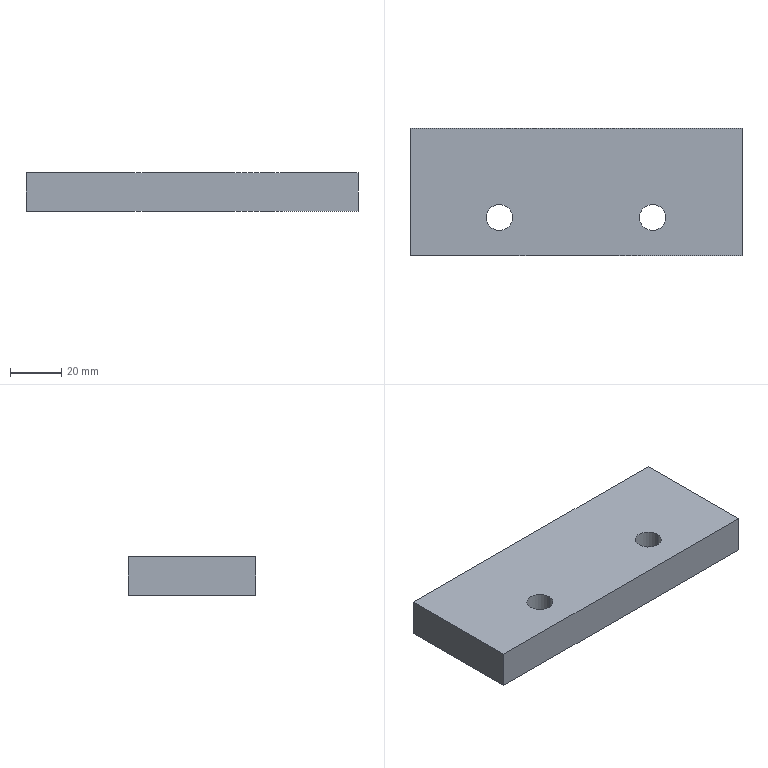Part | SolidWorks | features Extrusion 1, HoleWzd 1 | 1 solid | 10 faces | box 130 x 50 x 15 mm | volume 95049 mm3 | plane 6 | cylinder 4 | commonest cylinder face diameters 10.2 x4
STEP:
#1=CARTESIAN_POINT('',(-35.1,-10.,0.));
#2=VERTEX_POINT('',#1);
#3=CARTESIAN_POINT('',(-24.9,-10.,0.));
#4=VERTEX_POINT('',#3);
#5=CARTESIAN_POINT('',(-30.,-10.,0.));
#6=DIRECTION('',(0.,0.,1.));
#7=DIRECTION('',(1.,0.,0.));
#8=AXIS2_PLACEMENT_3D('',#5,#6,#7);
#9=CIRCLE('',#8,5.1);
#10=EDGE_CURVE('',#2,#4,#9,.T.);
#11=ORIENTED_EDGE('',*,*,#10,.F.);
#12=CARTESIAN_POINT('',(-35.1,-10.,15.));
#13=VERTEX_POINT('',#12);
#14=CARTESIAN_POINT('',(-35.1,-10.,15.));
#15=DIRECTION('',(0.,0.,1.));
#16=VECTOR('',#15,1000.);
#17=LINE('',#14,#16);
#18=EDGE_CURVE('',#2,#13,#17,.T.);
#19=ORIENTED_EDGE('',*,*,#18,.T.);
#20=CARTESIAN_POINT('',(-24.9,-10.,15.));
#21=VERTEX_POINT('',#20);
#22=CARTESIAN_POINT('',(-30.,-10.,15.));
#23=DIRECTION('',(0.,0.,1.));
#24=DIRECTION('',(1.,0.,0.));
#25=AXIS2_PLACEMENT_3D('',#22,#23,#24);
#26=CIRCLE('',#25,5.1);
#27=EDGE_CURVE('',#13,#21,#26,.T.);
#28=ORIENTED_EDGE('',*,*,#27,.T.);
#29=CARTESIAN_POINT('',(-24.9,-10.,15.));
#30=DIRECTION('',(0.,0.,1.));
#31=VECTOR('',#30,1000.);
#32=LINE('',#29,#31);
#33=EDGE_CURVE('',#4,#21,#32,.T.);
#34=ORIENTED_EDGE('',*,*,#33,.F.);
#35=EDGE_LOOP('',(#11,#19,#28,#34));
#36=FACE_OUTER_BOUND('',#35,.T.);
#37=CARTESIAN_POINT('',(-30.,-10.,15.));
#38=DIRECTION('',(0.,0.,1.));
#39=DIRECTION('',(1.,0.,0.));
#40=AXIS2_PLACEMENT_3D('',#37,#38,#39);
#41=CYLINDRICAL_SURFACE('',#40,5.1);
#42=ADVANCED_FACE('',(#36),#41,.F.);
#43=CARTESIAN_POINT('',(24.9,-10.,0.));
#44=VERTEX_POINT('',#43);
#45=CARTESIAN_POINT('',(35.1,-10.,0.));
#46=VERTEX_POINT('',#45);
#47=CARTESIAN_POINT('',(30.,-10.,0.));
#48=DIRECTION('',(0.,0.,1.));
#49=DIRECTION('',(1.,0.,0.));
#50=AXIS2_PLACEMENT_3D('',#47,#48,#49);
#51=CIRCLE('',#50,5.1);
#52=EDGE_CURVE('',#44,#46,#51,.T.);
#53=ORIENTED_EDGE('',*,*,#52,.F.);
#54=CARTESIAN_POINT('',(24.9,-10.,15.));
#55=VERTEX_POINT('',#54);
#56=CARTESIAN_POINT('',(24.9,-10.,15.));
#57=DIRECTION('',(0.,0.,1.));
#58=VECTOR('',#57,1000.);
#59=LINE('',#56,#58);
#60=EDGE_CURVE('',#44,#55,#59,.T.);
#61=ORIENTED_EDGE('',*,*,#60,.T.);
#62=CARTESIAN_POINT('',(35.1,-10.,15.));
#63=VERTEX_POINT('',#62);
#64=CARTESIAN_POINT('',(30.,-10.,15.));
#65=DIRECTION('',(0.,0.,1.));
#66=DIRECTION('',(1.,0.,0.));
#67=AXIS2_PLACEMENT_3D('',#64,#65,#66);
#68=CIRCLE('',#67,5.1);
#69=EDGE_CURVE('',#55,#63,#68,.T.);
#70=ORIENTED_EDGE('',*,*,#69,.T.);
#71=CARTESIAN_POINT('',(35.1,-10.,15.));
#72=DIRECTION('',(0.,0.,1.));
#73=VECTOR('',#72,1000.);
#74=LINE('',#71,#73);
#75=EDGE_CURVE('',#46,#63,#74,.T.);
#76=ORIENTED_EDGE('',*,*,#75,.F.);
#77=EDGE_LOOP('',(#53,#61,#70,#76));
#78=FACE_OUTER_BOUND('',#77,.T.);
#79=CARTESIAN_POINT('',(30.,-10.,15.));
#80=DIRECTION('',(0.,0.,1.));
#81=DIRECTION('',(1.,0.,0.));
#82=AXIS2_PLACEMENT_3D('',#79,#80,#81);
#83=CYLINDRICAL_SURFACE('',#82,5.1);
#84=ADVANCED_FACE('',(#78),#83,.F.);
#85=CARTESIAN_POINT('',(65.,-25.,0.));
#86=VERTEX_POINT('',#85);
#87=CARTESIAN_POINT('',(65.,25.,0.));
#88=VERTEX_POINT('',#87);
#89=CARTESIAN_POINT('',(65.,25.,0.));
#90=DIRECTION('',(0.,1.,0.));
#91=VECTOR('',#90,1000.);
#92=LINE('',#89,#91);
#93=EDGE_CURVE('',#86,#88,#92,.T.);
#94=ORIENTED_EDGE('',*,*,#93,.T.);
#95=CARTESIAN_POINT('',(65.,25.,15.));
#96=VERTEX_POINT('',#95);
#97=CARTESIAN_POINT('',(65.,25.,15.));
#98=DIRECTION('',(0.,0.,-1.));
#99=VECTOR('',#98,1000.);
#100=LINE('',#97,#99);
#101=EDGE_CURVE('',#96,#88,#100,.T.);
#102=ORIENTED_EDGE('',*,*,#101,.F.);
#103=CARTESIAN_POINT('',(65.,-25.,15.));
#104=VERTEX_POINT('',#103);
#105=CARTESIAN_POINT('',(65.,25.,15.));
#106=DIRECTION('',(0.,1.,0.));
#107=VECTOR('',#106,1000.);
#108=LINE('',#105,#107);
#109=EDGE_CURVE('',#104,#96,#108,.T.);
#110=ORIENTED_EDGE('',*,*,#109,.F.);
#111=CARTESIAN_POINT('',(65.,-25.,15.));
#112=DIRECTION('',(0.,0.,-1.));
#113=VECTOR('',#112,1000.);
#114=LINE('',#111,#113);
#115=EDGE_CURVE('',#104,#86,#114,.T.);
#116=ORIENTED_EDGE('',*,*,#115,.T.);
#117=EDGE_LOOP('',(#94,#102,#110,#116));
#118=FACE_OUTER_BOUND('',#117,.T.);
#119=CARTESIAN_POINT('',(65.,25.,15.));
#120=DIRECTION('',(-1.,0.,0.));
#121=DIRECTION('',(0.,0.,1.));
#122=AXIS2_PLACEMENT_3D('',#119,#120,#121);
#123=PLANE('',#122);
#124=ADVANCED_FACE('',(#118),#123,.F.);
#125=CARTESIAN_POINT('',(-65.,25.,0.));
#126=VERTEX_POINT('',#125);
#127=CARTESIAN_POINT('',(-65.,25.,0.));
#128=DIRECTION('',(-1.,0.,0.));
#129=VECTOR('',#128,1000.);
#130=LINE('',#127,#129);
#131=EDGE_CURVE('',#88,#126,#130,.T.);
#132=ORIENTED_EDGE('',*,*,#131,.T.);
#133=CARTESIAN_POINT('',(-65.,25.,15.));
#134=VERTEX_POINT('',#133);
#135=CARTESIAN_POINT('',(-65.,25.,15.));
#136=DIRECTION('',(0.,0.,-1.));
#137=VECTOR('',#136,1000.);
#138=LINE('',#135,#137);
#139=EDGE_CURVE('',#134,#126,#138,.T.);
#140=ORIENTED_EDGE('',*,*,#139,.F.);
#141=CARTESIAN_POINT('',(-65.,25.,15.));
#142=DIRECTION('',(-1.,0.,0.));
#143=VECTOR('',#142,1000.);
#144=LINE('',#141,#143);
#145=EDGE_CURVE('',#96,#134,#144,.T.);
#146=ORIENTED_EDGE('',*,*,#145,.F.);
#147=ORIENTED_EDGE('',*,*,#101,.T.);
#148=EDGE_LOOP('',(#132,#140,#146,#147));
#149=FACE_OUTER_BOUND('',#148,.T.);
#150=CARTESIAN_POINT('',(-65.,25.,15.));
#151=DIRECTION('',(0.,-1.,0.));
#152=DIRECTION('',(0.,0.,-1.));
#153=AXIS2_PLACEMENT_3D('',#150,#151,#152);
#154=PLANE('',#153);
#155=ADVANCED_FACE('',(#149),#154,.F.);
#156=CARTESIAN_POINT('',(-65.,-25.,0.));
#157=VERTEX_POINT('',#156);
#158=CARTESIAN_POINT('',(-65.,25.,0.));
#159=DIRECTION('',(0.,-1.,0.));
#160=VECTOR('',#159,1000.);
#161=LINE('',#158,#160);
#162=EDGE_CURVE('',#126,#157,#161,.T.);
#163=ORIENTED_EDGE('',*,*,#162,.T.);
#164=CARTESIAN_POINT('',(-65.,-25.,15.));
#165=VERTEX_POINT('',#164);
#166=CARTESIAN_POINT('',(-65.,-25.,15.));
#167=DIRECTION('',(0.,0.,-1.));
#168=VECTOR('',#167,1000.);
#169=LINE('',#166,#168);
#170=EDGE_CURVE('',#165,#157,#169,.T.);
#171=ORIENTED_EDGE('',*,*,#170,.F.);
#172=CARTESIAN_POINT('',(-65.,25.,15.));
#173=DIRECTION('',(0.,-1.,0.));
#174=VECTOR('',#173,1000.);
#175=LINE('',#172,#174);
#176=EDGE_CURVE('',#134,#165,#175,.T.);
#177=ORIENTED_EDGE('',*,*,#176,.F.);
#178=ORIENTED_EDGE('',*,*,#139,.T.);
#179=EDGE_LOOP('',(#163,#171,#177,#178));
#180=FACE_OUTER_BOUND('',#179,.T.);
#181=CARTESIAN_POINT('',(-65.,25.,15.));
#182=DIRECTION('',(1.,0.,0.));
#183=DIRECTION('',(0.,1.,0.));
#184=AXIS2_PLACEMENT_3D('',#181,#182,#183);
#185=PLANE('',#184);
#186=ADVANCED_FACE('',(#180),#185,.F.);
#187=CARTESIAN_POINT('',(-65.,-25.,0.));
#188=DIRECTION('',(1.,0.,0.));
#189=VECTOR('',#188,1000.);
#190=LINE('',#187,#189);
#191=EDGE_CURVE('',#157,#86,#190,.T.);
#192=ORIENTED_EDGE('',*,*,#191,.T.);
#193=ORIENTED_EDGE('',*,*,#115,.F.);
#194=CARTESIAN_POINT('',(-65.,-25.,15.));
#195=DIRECTION('',(1.,0.,0.));
#196=VECTOR('',#195,1000.);
#197=LINE('',#194,#196);
#198=EDGE_CURVE('',#165,#104,#197,.T.);
#199=ORIENTED_EDGE('',*,*,#198,.F.);
#200=ORIENTED_EDGE('',*,*,#170,.T.);
#201=EDGE_LOOP('',(#192,#193,#199,#200));
#202=FACE_OUTER_BOUND('',#201,.T.);
#203=CARTESIAN_POINT('',(-65.,-25.,15.));
#204=DIRECTION('',(0.,1.,0.));
#205=DIRECTION('',(0.,0.,1.));
#206=AXIS2_PLACEMENT_3D('',#203,#204,#205);
#207=PLANE('',#206);
#208=ADVANCED_FACE('',(#202),#207,.F.);
#209=CARTESIAN_POINT('',(-30.,-10.,15.));
#210=DIRECTION('',(0.,0.,1.));
#211=DIRECTION('',(1.,0.,0.));
#212=AXIS2_PLACEMENT_3D('',#209,#210,#211);
#213=CIRCLE('',#212,5.1);
#214=EDGE_CURVE('',#21,#13,#213,.T.);
#215=ORIENTED_EDGE('',*,*,#214,.F.);
#216=ORIENTED_EDGE('',*,*,#27,.F.);
#217=EDGE_LOOP('',(#215,#216));
#218=FACE_BOUND('',#217,.T.);
#219=CARTESIAN_POINT('',(30.,-10.,15.));
#220=DIRECTION('',(0.,0.,1.));
#221=DIRECTION('',(1.,0.,0.));
#222=AXIS2_PLACEMENT_3D('',#219,#220,#221);
#223=CIRCLE('',#222,5.1);
#224=EDGE_CURVE('',#63,#55,#223,.T.);
#225=ORIENTED_EDGE('',*,*,#224,.F.);
#226=ORIENTED_EDGE('',*,*,#69,.F.);
#227=EDGE_LOOP('',(#225,#226));
#228=FACE_BOUND('',#227,.T.);
#229=ORIENTED_EDGE('',*,*,#109,.T.);
#230=ORIENTED_EDGE('',*,*,#145,.T.);
#231=ORIENTED_EDGE('',*,*,#176,.T.);
#232=ORIENTED_EDGE('',*,*,#198,.T.);
#233=EDGE_LOOP('',(#229,#230,#231,#232));
#234=FACE_OUTER_BOUND('',#233,.T.);
#235=CARTESIAN_POINT('',(0.,0.,15.));
#236=DIRECTION('',(0.,0.,1.));
#237=DIRECTION('',(1.,0.,0.));
#238=AXIS2_PLACEMENT_3D('',#235,#236,#237);
#239=PLANE('',#238);
#240=ADVANCED_FACE('',(#218,#228,#234),#239,.T.);
#241=CARTESIAN_POINT('',(-30.,-10.,0.));
#242=DIRECTION('',(0.,0.,1.));
#243=DIRECTION('',(1.,0.,0.));
#244=AXIS2_PLACEMENT_3D('',#241,#242,#243);
#245=CIRCLE('',#244,5.1);
#246=EDGE_CURVE('',#4,#2,#245,.T.);
#247=ORIENTED_EDGE('',*,*,#246,.T.);
#248=ORIENTED_EDGE('',*,*,#10,.T.);
#249=EDGE_LOOP('',(#247,#248));
#250=FACE_BOUND('',#249,.T.);
#251=CARTESIAN_POINT('',(30.,-10.,0.));
#252=DIRECTION('',(0.,0.,1.));
#253=DIRECTION('',(1.,0.,0.));
#254=AXIS2_PLACEMENT_3D('',#251,#252,#253);
#255=CIRCLE('',#254,5.1);
#256=EDGE_CURVE('',#46,#44,#255,.T.);
#257=ORIENTED_EDGE('',*,*,#256,.T.);
#258=ORIENTED_EDGE('',*,*,#52,.T.);
#259=EDGE_LOOP('',(#257,#258));
#260=FACE_BOUND('',#259,.T.);
#261=ORIENTED_EDGE('',*,*,#93,.F.);
#262=ORIENTED_EDGE('',*,*,#191,.F.);
#263=ORIENTED_EDGE('',*,*,#162,.F.);
#264=ORIENTED_EDGE('',*,*,#131,.F.);
#265=EDGE_LOOP('',(#261,#262,#263,#264));
#266=FACE_OUTER_BOUND('',#265,.T.);
#267=CARTESIAN_POINT('',(0.,0.,0.));
#268=DIRECTION('',(0.,0.,1.));
#269=DIRECTION('',(1.,0.,0.));
#270=AXIS2_PLACEMENT_3D('',#267,#268,#269);
#271=PLANE('',#270);
#272=ADVANCED_FACE('',(#250,#260,#266),#271,.F.);
#273=ORIENTED_EDGE('',*,*,#60,.F.);
#274=ORIENTED_EDGE('',*,*,#256,.F.);
#275=ORIENTED_EDGE('',*,*,#75,.T.);
#276=ORIENTED_EDGE('',*,*,#224,.T.);
#277=EDGE_LOOP('',(#273,#274,#275,#276));
#278=FACE_OUTER_BOUND('',#277,.T.);
#279=CARTESIAN_POINT('',(30.,-10.,15.));
#280=DIRECTION('',(0.,0.,1.));
#281=DIRECTION('',(1.,0.,0.));
#282=AXIS2_PLACEMENT_3D('',#279,#280,#281);
#283=CYLINDRICAL_SURFACE('',#282,5.1);
#284=ADVANCED_FACE('',(#278),#283,.F.);
#285=ORIENTED_EDGE('',*,*,#18,.F.);
#286=ORIENTED_EDGE('',*,*,#246,.F.);
#287=ORIENTED_EDGE('',*,*,#33,.T.);
#288=ORIENTED_EDGE('',*,*,#214,.T.);
#289=EDGE_LOOP('',(#285,#286,#287,#288));
#290=FACE_OUTER_BOUND('',#289,.T.);
#291=CARTESIAN_POINT('',(-30.,-10.,15.));
#292=DIRECTION('',(0.,0.,1.));
#293=DIRECTION('',(1.,0.,0.));
#294=AXIS2_PLACEMENT_3D('',#291,#292,#293);
#295=CYLINDRICAL_SURFACE('',#294,5.1);
#296=ADVANCED_FACE('',(#290),#295,.F.);
#297=CLOSED_SHELL('',(#42,#84,#124,#155,#186,#208,#240,#272,#284,#296));
#298=MANIFOLD_SOLID_BREP('',#297);
#299=CARTESIAN_POINT('',(0.,0.,0.));
#300=DIRECTION('',(0.,0.,1.));
#301=DIRECTION('',(1.,0.,0.));
#302=AXIS2_PLACEMENT_3D('',#299,#300,#301);
#303=(LENGTH_UNIT()NAMED_UNIT(*)SI_UNIT(.MILLI.,.METRE.));
#304=UNCERTAINTY_MEASURE_WITH_UNIT(LENGTH_MEASURE(0.00001),#303,'','');
#305=(NAMED_UNIT(*)PLANE_ANGLE_UNIT()SI_UNIT($,.RADIAN.));
#306=(NAMED_UNIT(*)SI_UNIT($,.STERADIAN.)SOLID_ANGLE_UNIT());
#307=(GEOMETRIC_REPRESENTATION_CONTEXT(3)GLOBAL_UNCERTAINTY_ASSIGNED_CONTEXT((#304))GLOBAL_UNIT_ASSIGNED_CONTEXT((#303,#305,#306))REPRESENTATION_CONTEXT('',''));
#308=ADVANCED_BREP_SHAPE_REPRESENTATION('',(#298,#302),#307);